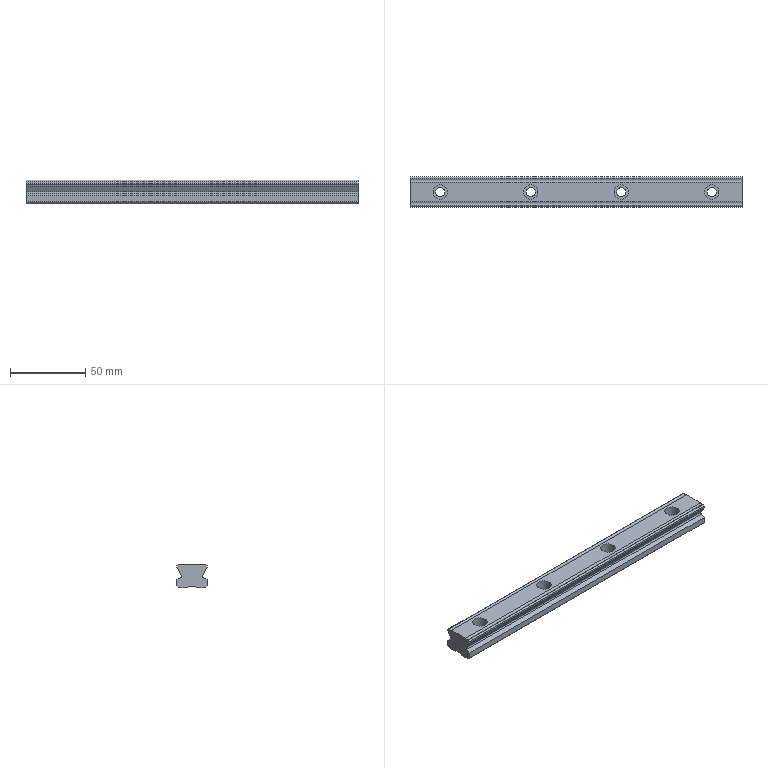Part | NX | 1 solid | 54 faces | box 220 x 20 x 15.5 mm | volume 57279 mm3 | plane 32 | cylinder 22 | commonest cylinder face diameters 6 x8 9.5 x8 2 x2 3.299 x2 3.3 x2